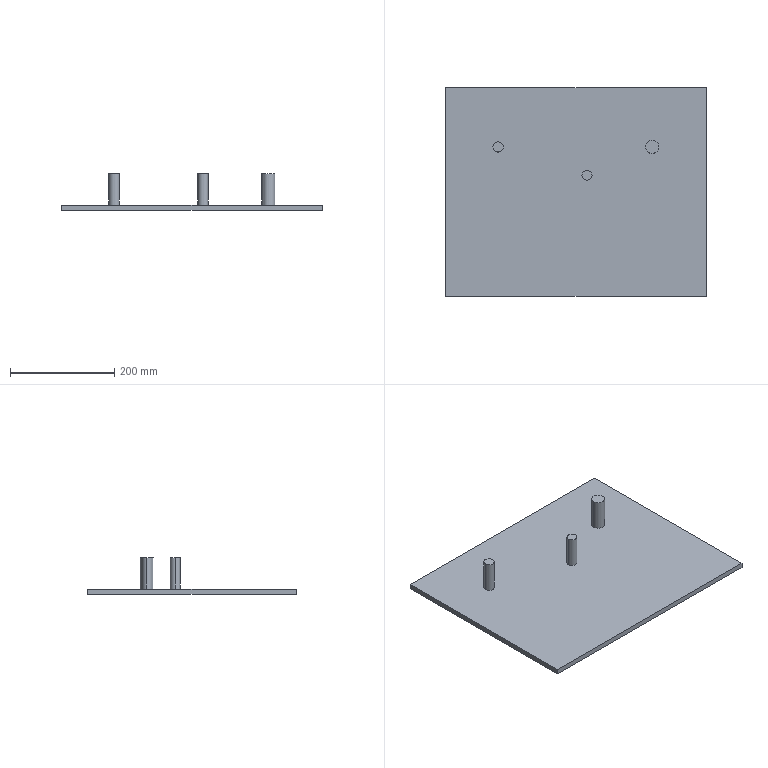Part | STEP file | MYT-A01-P34 | 1 solid | 15 faces | box 500 x 400 x 70 mm | volume 2065250 mm3 | plane 9 | cylinder 6 | commonest cylinder face diameters 19.238 x2 19.729 x2 25.007 x2
STEP:
#1=CARTESIAN_POINT('',(158.626,86.368,70.));
#2=VERTEX_POINT('',#1);
#3=CARTESIAN_POINT('',(133.619,86.368,70.));
#4=VERTEX_POINT('',#3);
#5=CARTESIAN_POINT('',(146.122,86.368,70.));
#6=DIRECTION('',(0.,0.,1.));
#7=DIRECTION('',(1.,0.,0.));
#8=AXIS2_PLACEMENT_3D('',#5,#6,#7);
#9=CIRCLE('',#8,12.503);
#10=EDGE_CURVE('',#2,#4,#9,.T.);
#11=ORIENTED_EDGE('',*,*,#10,.F.);
#12=CARTESIAN_POINT('',(158.626,86.368,10.));
#13=VERTEX_POINT('',#12);
#14=CARTESIAN_POINT('',(158.626,86.368,70.));
#15=DIRECTION('',(0.,0.,-1.));
#16=VECTOR('',#15,1000.);
#17=LINE('',#14,#16);
#18=EDGE_CURVE('',#2,#13,#17,.T.);
#19=ORIENTED_EDGE('',*,*,#18,.T.);
#20=CARTESIAN_POINT('',(133.619,86.368,10.));
#21=VERTEX_POINT('',#20);
#22=CARTESIAN_POINT('',(146.122,86.368,10.));
#23=DIRECTION('',(0.,0.,1.));
#24=DIRECTION('',(1.,0.,0.));
#25=AXIS2_PLACEMENT_3D('',#22,#23,#24);
#26=CIRCLE('',#25,12.503);
#27=EDGE_CURVE('',#13,#21,#26,.T.);
#28=ORIENTED_EDGE('',*,*,#27,.T.);
#29=CARTESIAN_POINT('',(133.619,86.368,70.));
#30=DIRECTION('',(0.,0.,-1.));
#31=VECTOR('',#30,1000.);
#32=LINE('',#29,#31);
#33=EDGE_CURVE('',#4,#21,#32,.T.);
#34=ORIENTED_EDGE('',*,*,#33,.F.);
#35=EDGE_LOOP('',(#11,#19,#28,#34));
#36=FACE_OUTER_BOUND('',#35,.T.);
#37=CARTESIAN_POINT('',(146.122,86.368,70.));
#38=DIRECTION('',(0.,0.,-1.));
#39=DIRECTION('',(-1.,0.,0.));
#40=AXIS2_PLACEMENT_3D('',#37,#38,#39);
#41=CYLINDRICAL_SURFACE('',#40,12.503);
#42=ADVANCED_FACE('',(#36),#41,.T.);
#43=CARTESIAN_POINT('',(30.702,32.058,70.));
#44=VERTEX_POINT('',#43);
#45=CARTESIAN_POINT('',(11.464,32.058,70.));
#46=VERTEX_POINT('',#45);
#47=CARTESIAN_POINT('',(21.083,32.058,70.));
#48=DIRECTION('',(0.,0.,1.));
#49=DIRECTION('',(1.,0.,0.));
#50=AXIS2_PLACEMENT_3D('',#47,#48,#49);
#51=CIRCLE('',#50,9.619);
#52=EDGE_CURVE('',#44,#46,#51,.T.);
#53=ORIENTED_EDGE('',*,*,#52,.F.);
#54=CARTESIAN_POINT('',(30.702,32.058,10.));
#55=VERTEX_POINT('',#54);
#56=CARTESIAN_POINT('',(30.702,32.058,70.));
#57=DIRECTION('',(0.,0.,-1.));
#58=VECTOR('',#57,1000.);
#59=LINE('',#56,#58);
#60=EDGE_CURVE('',#44,#55,#59,.T.);
#61=ORIENTED_EDGE('',*,*,#60,.T.);
#62=CARTESIAN_POINT('',(11.464,32.058,10.));
#63=VERTEX_POINT('',#62);
#64=CARTESIAN_POINT('',(21.083,32.058,10.));
#65=DIRECTION('',(0.,0.,1.));
#66=DIRECTION('',(1.,0.,0.));
#67=AXIS2_PLACEMENT_3D('',#64,#65,#66);
#68=CIRCLE('',#67,9.619);
#69=EDGE_CURVE('',#55,#63,#68,.T.);
#70=ORIENTED_EDGE('',*,*,#69,.T.);
#71=CARTESIAN_POINT('',(11.464,32.058,70.));
#72=DIRECTION('',(0.,0.,-1.));
#73=VECTOR('',#72,1000.);
#74=LINE('',#71,#73);
#75=EDGE_CURVE('',#46,#63,#74,.T.);
#76=ORIENTED_EDGE('',*,*,#75,.F.);
#77=EDGE_LOOP('',(#53,#61,#70,#76));
#78=FACE_OUTER_BOUND('',#77,.T.);
#79=CARTESIAN_POINT('',(21.083,32.058,70.));
#80=DIRECTION('',(0.,0.,-1.));
#81=DIRECTION('',(-1.,0.,0.));
#82=AXIS2_PLACEMENT_3D('',#79,#80,#81);
#83=CYLINDRICAL_SURFACE('',#82,9.619);
#84=ADVANCED_FACE('',(#78),#83,.T.);
#85=CARTESIAN_POINT('',(-139.561,86.368,70.));
#86=VERTEX_POINT('',#85);
#87=CARTESIAN_POINT('',(-159.29,86.368,70.));
#88=VERTEX_POINT('',#87);
#89=CARTESIAN_POINT('',(-149.425,86.368,70.));
#90=DIRECTION('',(0.,0.,1.));
#91=DIRECTION('',(1.,0.,0.));
#92=AXIS2_PLACEMENT_3D('',#89,#90,#91);
#93=CIRCLE('',#92,9.865);
#94=EDGE_CURVE('',#86,#88,#93,.T.);
#95=ORIENTED_EDGE('',*,*,#94,.F.);
#96=CARTESIAN_POINT('',(-139.561,86.368,10.));
#97=VERTEX_POINT('',#96);
#98=CARTESIAN_POINT('',(-139.561,86.368,70.));
#99=DIRECTION('',(0.,0.,-1.));
#100=VECTOR('',#99,1000.);
#101=LINE('',#98,#100);
#102=EDGE_CURVE('',#86,#97,#101,.T.);
#103=ORIENTED_EDGE('',*,*,#102,.T.);
#104=CARTESIAN_POINT('',(-159.29,86.368,10.));
#105=VERTEX_POINT('',#104);
#106=CARTESIAN_POINT('',(-149.425,86.368,10.));
#107=DIRECTION('',(0.,0.,1.));
#108=DIRECTION('',(1.,0.,0.));
#109=AXIS2_PLACEMENT_3D('',#106,#107,#108);
#110=CIRCLE('',#109,9.865);
#111=EDGE_CURVE('',#97,#105,#110,.T.);
#112=ORIENTED_EDGE('',*,*,#111,.T.);
#113=CARTESIAN_POINT('',(-159.29,86.368,70.));
#114=DIRECTION('',(0.,0.,-1.));
#115=VECTOR('',#114,1000.);
#116=LINE('',#113,#115);
#117=EDGE_CURVE('',#88,#105,#116,.T.);
#118=ORIENTED_EDGE('',*,*,#117,.F.);
#119=EDGE_LOOP('',(#95,#103,#112,#118));
#120=FACE_OUTER_BOUND('',#119,.T.);
#121=CARTESIAN_POINT('',(-149.425,86.368,70.));
#122=DIRECTION('',(0.,0.,-1.));
#123=DIRECTION('',(-1.,0.,0.));
#124=AXIS2_PLACEMENT_3D('',#121,#122,#123);
#125=CYLINDRICAL_SURFACE('',#124,9.865);
#126=ADVANCED_FACE('',(#120),#125,.T.);
#127=CARTESIAN_POINT('',(250.,-200.,0.));
#128=VERTEX_POINT('',#127);
#129=CARTESIAN_POINT('',(250.,200.,0.));
#130=VERTEX_POINT('',#129);
#131=CARTESIAN_POINT('',(250.,200.,0.));
#132=DIRECTION('',(0.,1.,0.));
#133=VECTOR('',#132,1000.);
#134=LINE('',#131,#133);
#135=EDGE_CURVE('',#128,#130,#134,.T.);
#136=ORIENTED_EDGE('',*,*,#135,.T.);
#137=CARTESIAN_POINT('',(250.,200.,10.));
#138=VERTEX_POINT('',#137);
#139=CARTESIAN_POINT('',(250.,200.,10.));
#140=DIRECTION('',(0.,0.,-1.));
#141=VECTOR('',#140,1000.);
#142=LINE('',#139,#141);
#143=EDGE_CURVE('',#138,#130,#142,.T.);
#144=ORIENTED_EDGE('',*,*,#143,.F.);
#145=CARTESIAN_POINT('',(250.,-200.,10.));
#146=VERTEX_POINT('',#145);
#147=CARTESIAN_POINT('',(250.,200.,10.));
#148=DIRECTION('',(0.,1.,0.));
#149=VECTOR('',#148,1000.);
#150=LINE('',#147,#149);
#151=EDGE_CURVE('',#146,#138,#150,.T.);
#152=ORIENTED_EDGE('',*,*,#151,.F.);
#153=CARTESIAN_POINT('',(250.,-200.,10.));
#154=DIRECTION('',(0.,0.,-1.));
#155=VECTOR('',#154,1000.);
#156=LINE('',#153,#155);
#157=EDGE_CURVE('',#146,#128,#156,.T.);
#158=ORIENTED_EDGE('',*,*,#157,.T.);
#159=EDGE_LOOP('',(#136,#144,#152,#158));
#160=FACE_OUTER_BOUND('',#159,.T.);
#161=CARTESIAN_POINT('',(250.,200.,10.));
#162=DIRECTION('',(-1.,0.,0.));
#163=DIRECTION('',(0.,-1.,0.));
#164=AXIS2_PLACEMENT_3D('',#161,#162,#163);
#165=PLANE('',#164);
#166=ADVANCED_FACE('',(#160),#165,.F.);
#167=CARTESIAN_POINT('',(-250.,200.,0.));
#168=VERTEX_POINT('',#167);
#169=CARTESIAN_POINT('',(-250.,200.,0.));
#170=DIRECTION('',(-1.,0.,0.));
#171=VECTOR('',#170,1000.);
#172=LINE('',#169,#171);
#173=EDGE_CURVE('',#130,#168,#172,.T.);
#174=ORIENTED_EDGE('',*,*,#173,.T.);
#175=CARTESIAN_POINT('',(-250.,200.,10.));
#176=VERTEX_POINT('',#175);
#177=CARTESIAN_POINT('',(-250.,200.,10.));
#178=DIRECTION('',(0.,0.,-1.));
#179=VECTOR('',#178,1000.);
#180=LINE('',#177,#179);
#181=EDGE_CURVE('',#176,#168,#180,.T.);
#182=ORIENTED_EDGE('',*,*,#181,.F.);
#183=CARTESIAN_POINT('',(-250.,200.,10.));
#184=DIRECTION('',(-1.,0.,0.));
#185=VECTOR('',#184,1000.);
#186=LINE('',#183,#185);
#187=EDGE_CURVE('',#138,#176,#186,.T.);
#188=ORIENTED_EDGE('',*,*,#187,.F.);
#189=ORIENTED_EDGE('',*,*,#143,.T.);
#190=EDGE_LOOP('',(#174,#182,#188,#189));
#191=FACE_OUTER_BOUND('',#190,.T.);
#192=CARTESIAN_POINT('',(-250.,200.,10.));
#193=DIRECTION('',(0.,-1.,0.));
#194=DIRECTION('',(0.,0.,-1.));
#195=AXIS2_PLACEMENT_3D('',#192,#193,#194);
#196=PLANE('',#195);
#197=ADVANCED_FACE('',(#191),#196,.F.);
#198=CARTESIAN_POINT('',(-250.,-200.,0.));
#199=VERTEX_POINT('',#198);
#200=CARTESIAN_POINT('',(-250.,200.,0.));
#201=DIRECTION('',(0.,-1.,0.));
#202=VECTOR('',#201,1000.);
#203=LINE('',#200,#202);
#204=EDGE_CURVE('',#168,#199,#203,.T.);
#205=ORIENTED_EDGE('',*,*,#204,.T.);
#206=CARTESIAN_POINT('',(-250.,-200.,10.));
#207=VERTEX_POINT('',#206);
#208=CARTESIAN_POINT('',(-250.,-200.,10.));
#209=DIRECTION('',(0.,0.,-1.));
#210=VECTOR('',#209,1000.);
#211=LINE('',#208,#210);
#212=EDGE_CURVE('',#207,#199,#211,.T.);
#213=ORIENTED_EDGE('',*,*,#212,.F.);
#214=CARTESIAN_POINT('',(-250.,200.,10.));
#215=DIRECTION('',(0.,-1.,0.));
#216=VECTOR('',#215,1000.);
#217=LINE('',#214,#216);
#218=EDGE_CURVE('',#176,#207,#217,.T.);
#219=ORIENTED_EDGE('',*,*,#218,.F.);
#220=ORIENTED_EDGE('',*,*,#181,.T.);
#221=EDGE_LOOP('',(#205,#213,#219,#220));
#222=FACE_OUTER_BOUND('',#221,.T.);
#223=CARTESIAN_POINT('',(-250.,200.,10.));
#224=DIRECTION('',(1.,0.,0.));
#225=DIRECTION('',(0.,1.,0.));
#226=AXIS2_PLACEMENT_3D('',#223,#224,#225);
#227=PLANE('',#226);
#228=ADVANCED_FACE('',(#222),#227,.F.);
#229=CARTESIAN_POINT('',(-250.,-200.,0.));
#230=DIRECTION('',(1.,0.,0.));
#231=VECTOR('',#230,1000.);
#232=LINE('',#229,#231);
#233=EDGE_CURVE('',#199,#128,#232,.T.);
#234=ORIENTED_EDGE('',*,*,#233,.T.);
#235=ORIENTED_EDGE('',*,*,#157,.F.);
#236=CARTESIAN_POINT('',(-250.,-200.,10.));
#237=DIRECTION('',(1.,0.,0.));
#238=VECTOR('',#237,1000.);
#239=LINE('',#236,#238);
#240=EDGE_CURVE('',#207,#146,#239,.T.);
#241=ORIENTED_EDGE('',*,*,#240,.F.);
#242=ORIENTED_EDGE('',*,*,#212,.T.);
#243=EDGE_LOOP('',(#234,#235,#241,#242));
#244=FACE_OUTER_BOUND('',#243,.T.);
#245=CARTESIAN_POINT('',(-250.,-200.,10.));
#246=DIRECTION('',(0.,1.,0.));
#247=DIRECTION('',(0.,0.,1.));
#248=AXIS2_PLACEMENT_3D('',#245,#246,#247);
#249=PLANE('',#248);
#250=ADVANCED_FACE('',(#244),#249,.F.);
#251=CARTESIAN_POINT('',(146.122,86.368,10.));
#252=DIRECTION('',(0.,0.,1.));
#253=DIRECTION('',(1.,0.,0.));
#254=AXIS2_PLACEMENT_3D('',#251,#252,#253);
#255=CIRCLE('',#254,12.503);
#256=EDGE_CURVE('',#21,#13,#255,.T.);
#257=ORIENTED_EDGE('',*,*,#256,.F.);
#258=ORIENTED_EDGE('',*,*,#27,.F.);
#259=EDGE_LOOP('',(#257,#258));
#260=FACE_BOUND('',#259,.T.);
#261=CARTESIAN_POINT('',(21.083,32.058,10.));
#262=DIRECTION('',(0.,0.,1.));
#263=DIRECTION('',(1.,0.,0.));
#264=AXIS2_PLACEMENT_3D('',#261,#262,#263);
#265=CIRCLE('',#264,9.619);
#266=EDGE_CURVE('',#63,#55,#265,.T.);
#267=ORIENTED_EDGE('',*,*,#266,.F.);
#268=ORIENTED_EDGE('',*,*,#69,.F.);
#269=EDGE_LOOP('',(#267,#268));
#270=FACE_BOUND('',#269,.T.);
#271=CARTESIAN_POINT('',(-149.425,86.368,10.));
#272=DIRECTION('',(0.,0.,1.));
#273=DIRECTION('',(1.,0.,0.));
#274=AXIS2_PLACEMENT_3D('',#271,#272,#273);
#275=CIRCLE('',#274,9.865);
#276=EDGE_CURVE('',#105,#97,#275,.T.);
#277=ORIENTED_EDGE('',*,*,#276,.F.);
#278=ORIENTED_EDGE('',*,*,#111,.F.);
#279=EDGE_LOOP('',(#277,#278));
#280=FACE_BOUND('',#279,.T.);
#281=ORIENTED_EDGE('',*,*,#151,.T.);
#282=ORIENTED_EDGE('',*,*,#187,.T.);
#283=ORIENTED_EDGE('',*,*,#218,.T.);
#284=ORIENTED_EDGE('',*,*,#240,.T.);
#285=EDGE_LOOP('',(#281,#282,#283,#284));
#286=FACE_OUTER_BOUND('',#285,.T.);
#287=CARTESIAN_POINT('',(0.,0.,10.));
#288=DIRECTION('',(0.,0.,1.));
#289=DIRECTION('',(1.,0.,0.));
#290=AXIS2_PLACEMENT_3D('',#287,#288,#289);
#291=PLANE('',#290);
#292=ADVANCED_FACE('',(#260,#270,#280,#286),#291,.T.);
#293=ORIENTED_EDGE('',*,*,#135,.F.);
#294=ORIENTED_EDGE('',*,*,#233,.F.);
#295=ORIENTED_EDGE('',*,*,#204,.F.);
#296=ORIENTED_EDGE('',*,*,#173,.F.);
#297=EDGE_LOOP('',(#293,#294,#295,#296));
#298=FACE_OUTER_BOUND('',#297,.T.);
#299=CARTESIAN_POINT('',(0.,0.,0.));
#300=DIRECTION('',(0.,0.,1.));
#301=DIRECTION('',(1.,0.,0.));
#302=AXIS2_PLACEMENT_3D('',#299,#300,#301);
#303=PLANE('',#302);
#304=ADVANCED_FACE('',(#298),#303,.F.);
#305=ORIENTED_EDGE('',*,*,#102,.F.);
#306=CARTESIAN_POINT('',(-149.425,86.368,70.));
#307=DIRECTION('',(0.,0.,1.));
#308=DIRECTION('',(1.,0.,0.));
#309=AXIS2_PLACEMENT_3D('',#306,#307,#308);
#310=CIRCLE('',#309,9.865);
#311=EDGE_CURVE('',#88,#86,#310,.T.);
#312=ORIENTED_EDGE('',*,*,#311,.F.);
#313=ORIENTED_EDGE('',*,*,#117,.T.);
#314=ORIENTED_EDGE('',*,*,#276,.T.);
#315=EDGE_LOOP('',(#305,#312,#313,#314));
#316=FACE_OUTER_BOUND('',#315,.T.);
#317=CARTESIAN_POINT('',(-149.425,86.368,70.));
#318=DIRECTION('',(0.,0.,-1.));
#319=DIRECTION('',(-1.,0.,0.));
#320=AXIS2_PLACEMENT_3D('',#317,#318,#319);
#321=CYLINDRICAL_SURFACE('',#320,9.865);
#322=ADVANCED_FACE('',(#316),#321,.T.);
#323=ORIENTED_EDGE('',*,*,#311,.T.);
#324=ORIENTED_EDGE('',*,*,#94,.T.);
#325=EDGE_LOOP('',(#323,#324));
#326=FACE_OUTER_BOUND('',#325,.T.);
#327=CARTESIAN_POINT('',(-149.425,86.368,70.));
#328=DIRECTION('',(0.,0.,1.));
#329=DIRECTION('',(1.,0.,0.));
#330=AXIS2_PLACEMENT_3D('',#327,#328,#329);
#331=PLANE('',#330);
#332=ADVANCED_FACE('',(#326),#331,.T.);
#333=ORIENTED_EDGE('',*,*,#60,.F.);
#334=CARTESIAN_POINT('',(21.083,32.058,70.));
#335=DIRECTION('',(0.,0.,1.));
#336=DIRECTION('',(1.,0.,0.));
#337=AXIS2_PLACEMENT_3D('',#334,#335,#336);
#338=CIRCLE('',#337,9.619);
#339=EDGE_CURVE('',#46,#44,#338,.T.);
#340=ORIENTED_EDGE('',*,*,#339,.F.);
#341=ORIENTED_EDGE('',*,*,#75,.T.);
#342=ORIENTED_EDGE('',*,*,#266,.T.);
#343=EDGE_LOOP('',(#333,#340,#341,#342));
#344=FACE_OUTER_BOUND('',#343,.T.);
#345=CARTESIAN_POINT('',(21.083,32.058,70.));
#346=DIRECTION('',(0.,0.,-1.));
#347=DIRECTION('',(-1.,0.,0.));
#348=AXIS2_PLACEMENT_3D('',#345,#346,#347);
#349=CYLINDRICAL_SURFACE('',#348,9.619);
#350=ADVANCED_FACE('',(#344),#349,.T.);
#351=ORIENTED_EDGE('',*,*,#339,.T.);
#352=ORIENTED_EDGE('',*,*,#52,.T.);
#353=EDGE_LOOP('',(#351,#352));
#354=FACE_OUTER_BOUND('',#353,.T.);
#355=CARTESIAN_POINT('',(21.083,32.058,70.));
#356=DIRECTION('',(0.,0.,1.));
#357=DIRECTION('',(1.,0.,0.));
#358=AXIS2_PLACEMENT_3D('',#355,#356,#357);
#359=PLANE('',#358);
#360=ADVANCED_FACE('',(#354),#359,.T.);
#361=ORIENTED_EDGE('',*,*,#18,.F.);
#362=CARTESIAN_POINT('',(146.122,86.368,70.));
#363=DIRECTION('',(0.,0.,1.));
#364=DIRECTION('',(1.,0.,0.));
#365=AXIS2_PLACEMENT_3D('',#362,#363,#364);
#366=CIRCLE('',#365,12.503);
#367=EDGE_CURVE('',#4,#2,#366,.T.);
#368=ORIENTED_EDGE('',*,*,#367,.F.);
#369=ORIENTED_EDGE('',*,*,#33,.T.);
#370=ORIENTED_EDGE('',*,*,#256,.T.);
#371=EDGE_LOOP('',(#361,#368,#369,#370));
#372=FACE_OUTER_BOUND('',#371,.T.);
#373=CARTESIAN_POINT('',(146.122,86.368,70.));
#374=DIRECTION('',(0.,0.,-1.));
#375=DIRECTION('',(-1.,0.,0.));
#376=AXIS2_PLACEMENT_3D('',#373,#374,#375);
#377=CYLINDRICAL_SURFACE('',#376,12.503);
#378=ADVANCED_FACE('',(#372),#377,.T.);
#379=ORIENTED_EDGE('',*,*,#367,.T.);
#380=ORIENTED_EDGE('',*,*,#10,.T.);
#381=EDGE_LOOP('',(#379,#380));
#382=FACE_OUTER_BOUND('',#381,.T.);
#383=CARTESIAN_POINT('',(146.122,86.368,70.));
#384=DIRECTION('',(0.,0.,1.));
#385=DIRECTION('',(1.,0.,0.));
#386=AXIS2_PLACEMENT_3D('',#383,#384,#385);
#387=PLANE('',#386);
#388=ADVANCED_FACE('',(#382),#387,.T.);
#389=CLOSED_SHELL('',(#42,#84,#126,#166,#197,#228,#250,#292,#304,#322,#332,#350,#360,#378,#388));
#390=MANIFOLD_SOLID_BREP('',#389);
#391=CARTESIAN_POINT('',(0.,0.,0.));
#392=DIRECTION('',(0.,0.,1.));
#393=DIRECTION('',(1.,0.,0.));
#394=AXIS2_PLACEMENT_3D('',#391,#392,#393);
#395=(LENGTH_UNIT()NAMED_UNIT(*)SI_UNIT(.MILLI.,.METRE.));
#396=UNCERTAINTY_MEASURE_WITH_UNIT(LENGTH_MEASURE(0.00001),#395,'','');
#397=(NAMED_UNIT(*)PLANE_ANGLE_UNIT()SI_UNIT($,.RADIAN.));
#398=(NAMED_UNIT(*)SI_UNIT($,.STERADIAN.)SOLID_ANGLE_UNIT());
#399=(GEOMETRIC_REPRESENTATION_CONTEXT(3)GLOBAL_UNCERTAINTY_ASSIGNED_CONTEXT((#396))GLOBAL_UNIT_ASSIGNED_CONTEXT((#395,#397,#398))REPRESENTATION_CONTEXT('',''));
#400=ADVANCED_BREP_SHAPE_REPRESENTATION('',(#390,#394),#399);